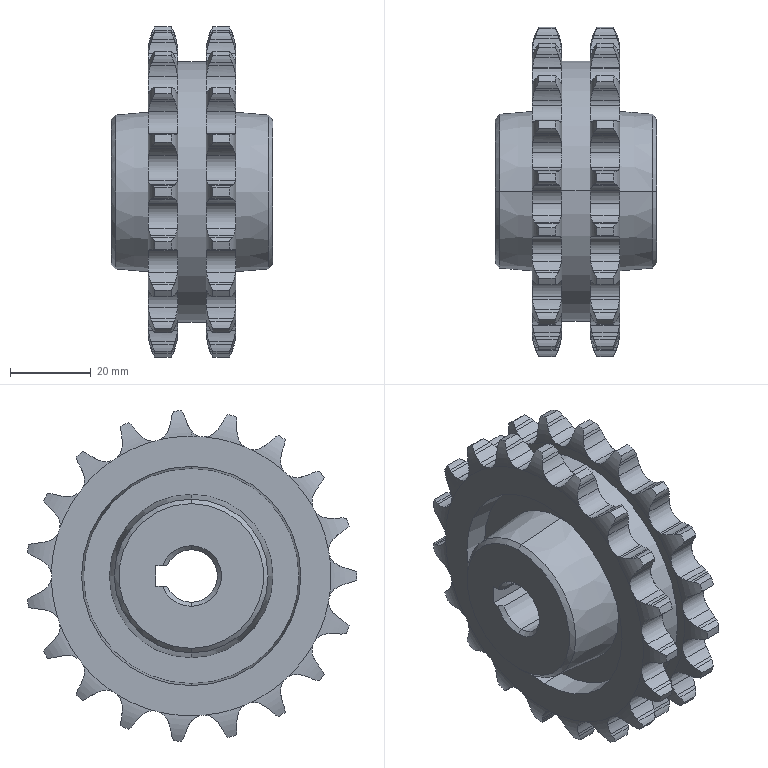Part | SolidWorks | features Cut 2, Revolution 2, Chamfer 1, CirPattern 1, LPattern 1 | 2 solids | 440 faces | box 40 x 81.595 x 81.862 mm | volume 92773 mm3 | cylinder 253 | plane 87 | torus 80 | cone 20 | commonest cylinder face diameters 11.518 x80 20.732 x80 8.06 x48 82 x38 13 x3 54.299 x2